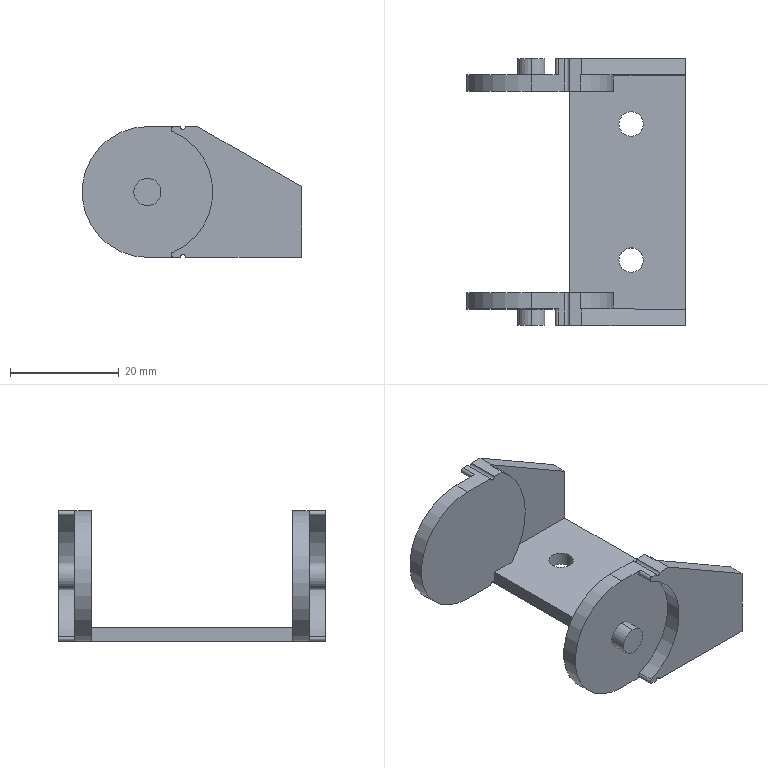Part | STEP file | 18_37_3 | 1 solid | 46 faces | box 40.3 x 49 x 24 mm | volume 7598 mm3 | cylinder 24 | plane 22 | commonest cylinder face diameters 1 x10 4.5 x4 5 x4 24 x4 30 x2